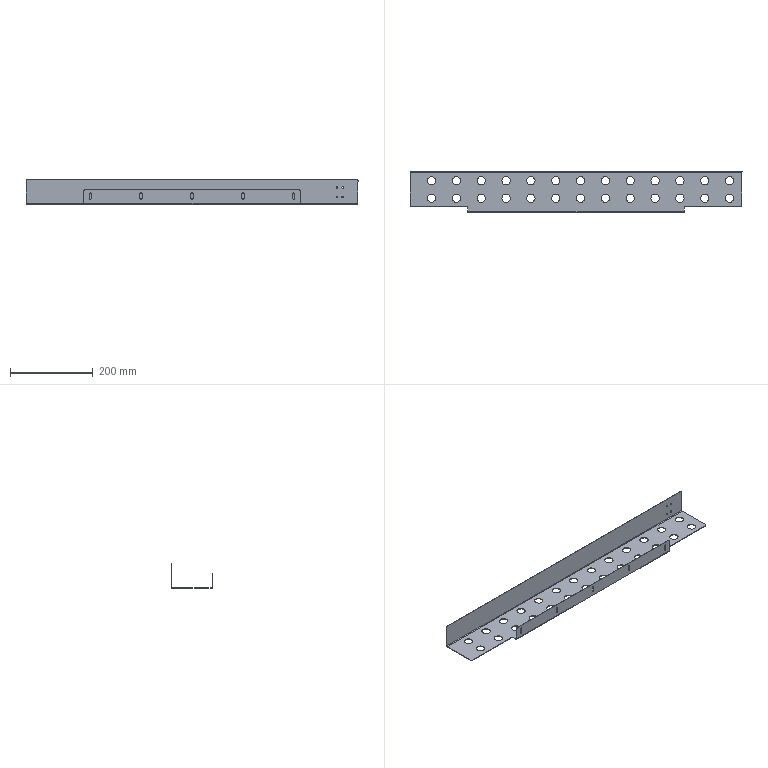Part | STEP file | SynoNew-0304-063 | 1 solid | 80 faces | box 802 x 100 x 60 mm | volume 195750 mm3 | cylinder 52 | plane 28 | commonest cylinder face diameters 20 x26 5.5 x10 6 x10 4.2 x4 3 x2